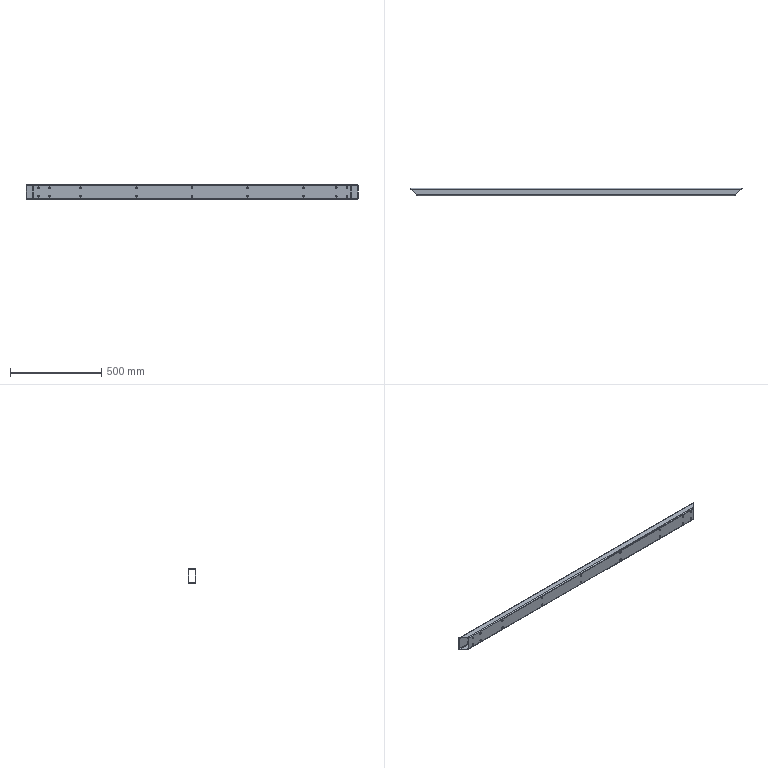Part | STEP file | SN10_002_008-01_TUBO_RETANGULAR | 1 solid | 54 faces | box 1820 x 40 x 80 mm | volume 1167783 mm3 | cylinder 44 | plane 10 | commonest cylinder face diameters 10 x36 6 x4 12 x4